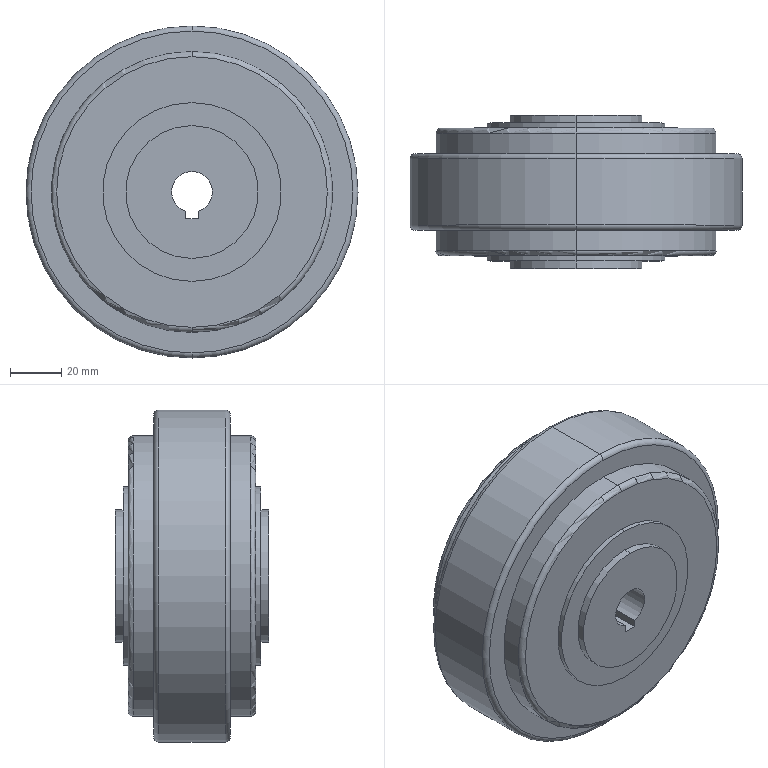Part | STEP file | 6NMMagnetic powder brake | 1 solid | 59 faces | box 130 x 60 x 130 mm | volume 601395 mm3 | cylinder 28 | cone 12 | plane 11 | torus 8 | commonest cylinder face diameters 4.2 x12 52 x4 70 x4 110 x4 16 x2 130 x2